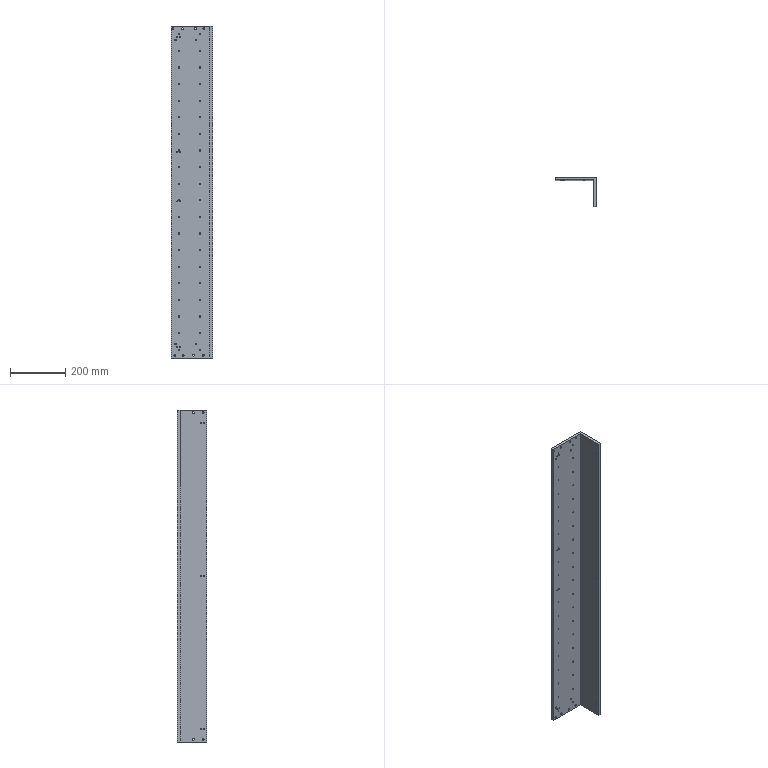Part | SolidWorks | features HoleWzd 7, Extrusion 1, MoveFace 1 | 1 solid | 148 faces | box 150 x 105 x 1200 mm | volume 2927452 mm3 | cylinder 140 | plane 8 | commonest cylinder face diameters 4.2 x80 6.8 x24 5 x20 3.3 x16